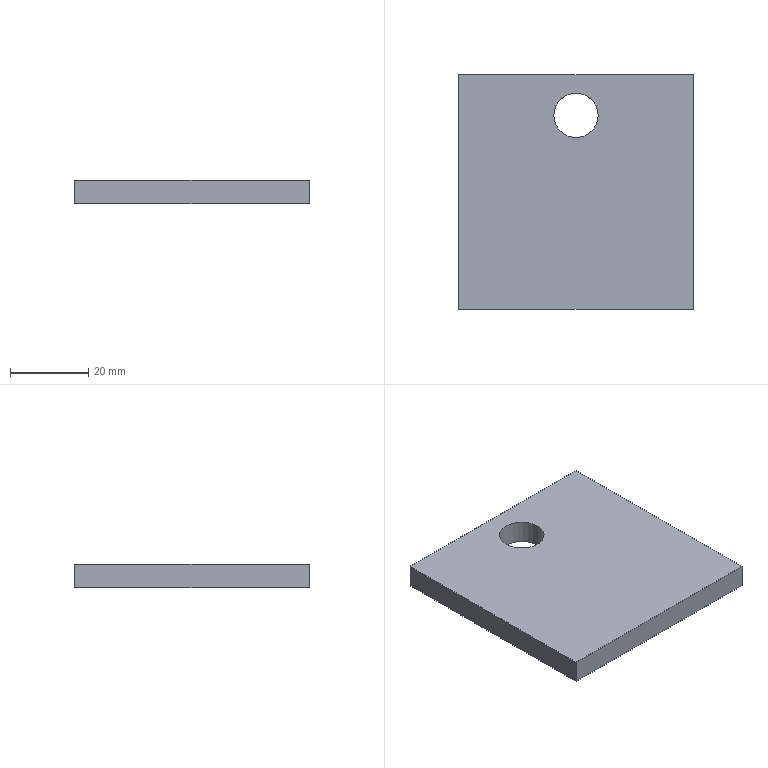Part | NX | features 凸台-拉伸21[1] 2 | 1 solid | 8 faces | box 60 x 60 x 6 mm | volume 20990 mm3 | plane 6 | cylinder 2 | commonest cylinder face diameters 11.377 x2
STEP:
#1=CARTESIAN_POINT('',(2757.312,-550.427,-1102.985));
#2=VERTEX_POINT('',#1);
#3=CARTESIAN_POINT('',(2757.312,-550.427,-1108.985));
#4=VERTEX_POINT('',#3);
#5=CARTESIAN_POINT('',(2757.312,-550.427,-1108.985));
#6=DIRECTION('',(0.,0.,1.));
#7=VECTOR('',#6,1000.);
#8=LINE('',#5,#7);
#9=EDGE_CURVE('',#2,#4,#8,.F.);
#10=ORIENTED_EDGE('',*,*,#9,.T.);
#11=CARTESIAN_POINT('',(2768.688,-550.427,-1108.985));
#12=VERTEX_POINT('',#11);
#13=CARTESIAN_POINT('',(2763.,-550.427,-1108.985));
#14=DIRECTION('',(0.,0.,-1.));
#15=DIRECTION('',(-1.,0.,0.));
#16=AXIS2_PLACEMENT_3D('',#13,#14,#15);
#17=CIRCLE('',#16,5.688);
#18=EDGE_CURVE('',#4,#12,#17,.T.);
#19=ORIENTED_EDGE('',*,*,#18,.T.);
#20=CARTESIAN_POINT('',(2768.688,-550.427,-1102.985));
#21=VERTEX_POINT('',#20);
#22=CARTESIAN_POINT('',(2768.688,-550.427,-1108.985));
#23=DIRECTION('',(0.,0.,1.));
#24=VECTOR('',#23,1000.);
#25=LINE('',#22,#24);
#26=EDGE_CURVE('',#12,#21,#25,.T.);
#27=ORIENTED_EDGE('',*,*,#26,.T.);
#28=CARTESIAN_POINT('',(2763.,-550.427,-1102.985));
#29=DIRECTION('',(0.,0.,-1.));
#30=DIRECTION('',(-1.,0.,0.));
#31=AXIS2_PLACEMENT_3D('',#28,#29,#30);
#32=CIRCLE('',#31,5.688);
#33=EDGE_CURVE('',#2,#21,#32,.T.);
#34=ORIENTED_EDGE('',*,*,#33,.F.);
#35=EDGE_LOOP('',(#10,#19,#27,#34));
#36=FACE_BOUND('',#35,.T.);
#37=CARTESIAN_POINT('',(2763.,-550.427,-1108.985));
#38=DIRECTION('',(0.,0.,1.));
#39=DIRECTION('',(1.,0.,0.));
#40=AXIS2_PLACEMENT_3D('',#37,#38,#39);
#41=CYLINDRICAL_SURFACE('',#40,5.688);
#42=ADVANCED_FACE('',(#36),#41,.F.);
#43=CARTESIAN_POINT('',(2733.,-540.,-1102.985));
#44=VERTEX_POINT('',#43);
#45=CARTESIAN_POINT('',(2793.,-540.,-1102.985));
#46=VERTEX_POINT('',#45);
#47=CARTESIAN_POINT('',(2793.,-540.,-1102.985));
#48=DIRECTION('',(1.,0.,0.));
#49=VECTOR('',#48,1000.);
#50=LINE('',#47,#49);
#51=EDGE_CURVE('',#44,#46,#50,.T.);
#52=ORIENTED_EDGE('',*,*,#51,.T.);
#53=CARTESIAN_POINT('',(2793.,-540.,-1108.985));
#54=VERTEX_POINT('',#53);
#55=CARTESIAN_POINT('',(2793.,-540.,-1108.985));
#56=DIRECTION('',(0.,0.,1.));
#57=VECTOR('',#56,1000.);
#58=LINE('',#55,#57);
#59=EDGE_CURVE('',#54,#46,#58,.T.);
#60=ORIENTED_EDGE('',*,*,#59,.F.);
#61=CARTESIAN_POINT('',(2733.,-540.,-1108.985));
#62=VERTEX_POINT('',#61);
#63=CARTESIAN_POINT('',(2793.,-540.,-1108.985));
#64=DIRECTION('',(1.,0.,0.));
#65=VECTOR('',#64,1000.);
#66=LINE('',#63,#65);
#67=EDGE_CURVE('',#62,#54,#66,.T.);
#68=ORIENTED_EDGE('',*,*,#67,.F.);
#69=CARTESIAN_POINT('',(2733.,-540.,-1108.985));
#70=DIRECTION('',(0.,0.,1.));
#71=VECTOR('',#70,1000.);
#72=LINE('',#69,#71);
#73=EDGE_CURVE('',#62,#44,#72,.T.);
#74=ORIENTED_EDGE('',*,*,#73,.T.);
#75=EDGE_LOOP('',(#52,#60,#68,#74));
#76=FACE_BOUND('',#75,.T.);
#77=CARTESIAN_POINT('',(2793.,-540.,-1108.985));
#78=DIRECTION('',(0.,-1.,0.));
#79=DIRECTION('',(0.,0.,-1.));
#80=AXIS2_PLACEMENT_3D('',#77,#78,#79);
#81=PLANE('',#80);
#82=ADVANCED_FACE('',(#76),#81,.F.);
#83=CARTESIAN_POINT('',(2733.,-600.,-1102.985));
#84=VERTEX_POINT('',#83);
#85=CARTESIAN_POINT('',(2733.,-600.,-1102.985));
#86=DIRECTION('',(0.,1.,0.));
#87=VECTOR('',#86,1000.);
#88=LINE('',#85,#87);
#89=EDGE_CURVE('',#84,#44,#88,.T.);
#90=ORIENTED_EDGE('',*,*,#89,.T.);
#91=ORIENTED_EDGE('',*,*,#73,.F.);
#92=CARTESIAN_POINT('',(2733.,-600.,-1108.985));
#93=VERTEX_POINT('',#92);
#94=CARTESIAN_POINT('',(2733.,-600.,-1108.985));
#95=DIRECTION('',(0.,1.,0.));
#96=VECTOR('',#95,1000.);
#97=LINE('',#94,#96);
#98=EDGE_CURVE('',#93,#62,#97,.T.);
#99=ORIENTED_EDGE('',*,*,#98,.F.);
#100=CARTESIAN_POINT('',(2733.,-600.,-1108.985));
#101=DIRECTION('',(0.,0.,1.));
#102=VECTOR('',#101,1000.);
#103=LINE('',#100,#102);
#104=EDGE_CURVE('',#93,#84,#103,.T.);
#105=ORIENTED_EDGE('',*,*,#104,.T.);
#106=EDGE_LOOP('',(#90,#91,#99,#105));
#107=FACE_BOUND('',#106,.T.);
#108=CARTESIAN_POINT('',(2733.,-600.,-1108.985));
#109=DIRECTION('',(1.,0.,0.));
#110=DIRECTION('',(0.,0.,-1.));
#111=AXIS2_PLACEMENT_3D('',#108,#109,#110);
#112=PLANE('',#111);
#113=ADVANCED_FACE('',(#107),#112,.F.);
#114=CARTESIAN_POINT('',(2793.,-600.,-1102.985));
#115=VERTEX_POINT('',#114);
#116=CARTESIAN_POINT('',(2793.,-600.,-1102.985));
#117=DIRECTION('',(-1.,0.,0.));
#118=VECTOR('',#117,1000.);
#119=LINE('',#116,#118);
#120=EDGE_CURVE('',#115,#84,#119,.T.);
#121=ORIENTED_EDGE('',*,*,#120,.T.);
#122=ORIENTED_EDGE('',*,*,#104,.F.);
#123=CARTESIAN_POINT('',(2793.,-600.,-1108.985));
#124=VERTEX_POINT('',#123);
#125=CARTESIAN_POINT('',(2793.,-600.,-1108.985));
#126=DIRECTION('',(-1.,0.,0.));
#127=VECTOR('',#126,1000.);
#128=LINE('',#125,#127);
#129=EDGE_CURVE('',#124,#93,#128,.T.);
#130=ORIENTED_EDGE('',*,*,#129,.F.);
#131=CARTESIAN_POINT('',(2793.,-600.,-1108.985));
#132=DIRECTION('',(0.,0.,1.));
#133=VECTOR('',#132,1000.);
#134=LINE('',#131,#133);
#135=EDGE_CURVE('',#124,#115,#134,.T.);
#136=ORIENTED_EDGE('',*,*,#135,.T.);
#137=EDGE_LOOP('',(#121,#122,#130,#136));
#138=FACE_BOUND('',#137,.T.);
#139=CARTESIAN_POINT('',(2793.,-600.,-1108.985));
#140=DIRECTION('',(0.,1.,0.));
#141=DIRECTION('',(0.,0.,1.));
#142=AXIS2_PLACEMENT_3D('',#139,#140,#141);
#143=PLANE('',#142);
#144=ADVANCED_FACE('',(#138),#143,.F.);
#145=CARTESIAN_POINT('',(2793.,-600.,-1102.985));
#146=DIRECTION('',(0.,-1.,0.));
#147=VECTOR('',#146,1000.);
#148=LINE('',#145,#147);
#149=EDGE_CURVE('',#46,#115,#148,.T.);
#150=ORIENTED_EDGE('',*,*,#149,.T.);
#151=ORIENTED_EDGE('',*,*,#135,.F.);
#152=CARTESIAN_POINT('',(2793.,-600.,-1108.985));
#153=DIRECTION('',(0.,-1.,0.));
#154=VECTOR('',#153,1000.);
#155=LINE('',#152,#154);
#156=EDGE_CURVE('',#54,#124,#155,.T.);
#157=ORIENTED_EDGE('',*,*,#156,.F.);
#158=ORIENTED_EDGE('',*,*,#59,.T.);
#159=EDGE_LOOP('',(#150,#151,#157,#158));
#160=FACE_BOUND('',#159,.T.);
#161=CARTESIAN_POINT('',(2793.,-600.,-1108.985));
#162=DIRECTION('',(-1.,0.,0.));
#163=DIRECTION('',(0.,0.,1.));
#164=AXIS2_PLACEMENT_3D('',#161,#162,#163);
#165=PLANE('',#164);
#166=ADVANCED_FACE('',(#160),#165,.F.);
#167=CARTESIAN_POINT('',(2763.,-550.427,-1102.985));
#168=DIRECTION('',(0.,0.,-1.));
#169=DIRECTION('',(-1.,0.,0.));
#170=AXIS2_PLACEMENT_3D('',#167,#168,#169);
#171=CIRCLE('',#170,5.688);
#172=EDGE_CURVE('',#21,#2,#171,.T.);
#173=ORIENTED_EDGE('',*,*,#172,.T.);
#174=ORIENTED_EDGE('',*,*,#33,.T.);
#175=EDGE_LOOP('',(#173,#174));
#176=FACE_BOUND('',#175,.T.);
#177=ORIENTED_EDGE('',*,*,#149,.F.);
#178=ORIENTED_EDGE('',*,*,#51,.F.);
#179=ORIENTED_EDGE('',*,*,#89,.F.);
#180=ORIENTED_EDGE('',*,*,#120,.F.);
#181=EDGE_LOOP('',(#177,#178,#179,#180));
#182=FACE_BOUND('',#181,.T.);
#183=CARTESIAN_POINT('',(1500.,0.,-1102.985));
#184=DIRECTION('',(0.,0.,1.));
#185=DIRECTION('',(1.,0.,0.));
#186=AXIS2_PLACEMENT_3D('',#183,#184,#185);
#187=PLANE('',#186);
#188=ADVANCED_FACE('',(#176,#182),#187,.T.);
#189=CARTESIAN_POINT('',(2763.,-550.427,-1108.985));
#190=DIRECTION('',(0.,0.,-1.));
#191=DIRECTION('',(-1.,0.,0.));
#192=AXIS2_PLACEMENT_3D('',#189,#190,#191);
#193=CIRCLE('',#192,5.688);
#194=EDGE_CURVE('',#12,#4,#193,.T.);
#195=ORIENTED_EDGE('',*,*,#194,.F.);
#196=ORIENTED_EDGE('',*,*,#18,.F.);
#197=EDGE_LOOP('',(#195,#196));
#198=FACE_BOUND('',#197,.T.);
#199=ORIENTED_EDGE('',*,*,#156,.T.);
#200=ORIENTED_EDGE('',*,*,#129,.T.);
#201=ORIENTED_EDGE('',*,*,#98,.T.);
#202=ORIENTED_EDGE('',*,*,#67,.T.);
#203=EDGE_LOOP('',(#199,#200,#201,#202));
#204=FACE_BOUND('',#203,.T.);
#205=CARTESIAN_POINT('',(1500.,0.,-1108.985));
#206=DIRECTION('',(0.,0.,1.));
#207=DIRECTION('',(1.,0.,0.));
#208=AXIS2_PLACEMENT_3D('',#205,#206,#207);
#209=PLANE('',#208);
#210=ADVANCED_FACE('',(#198,#204),#209,.F.);
#211=ORIENTED_EDGE('',*,*,#194,.T.);
#212=ORIENTED_EDGE('',*,*,#9,.F.);
#213=ORIENTED_EDGE('',*,*,#172,.F.);
#214=ORIENTED_EDGE('',*,*,#26,.F.);
#215=EDGE_LOOP('',(#211,#212,#213,#214));
#216=FACE_BOUND('',#215,.T.);
#217=CARTESIAN_POINT('',(2763.,-550.427,-1108.985));
#218=DIRECTION('',(0.,0.,1.));
#219=DIRECTION('',(1.,0.,0.));
#220=AXIS2_PLACEMENT_3D('',#217,#218,#219);
#221=CYLINDRICAL_SURFACE('',#220,5.688);
#222=ADVANCED_FACE('',(#216),#221,.F.);
#223=CLOSED_SHELL('',(#42,#82,#113,#144,#166,#188,#210,#222));
#224=MANIFOLD_SOLID_BREP('',#223);
#225=(LENGTH_UNIT()NAMED_UNIT(*)SI_UNIT(.MILLI.,.METRE.));
#226=UNCERTAINTY_MEASURE_WITH_UNIT(LENGTH_MEASURE(0.00001),#225,'','');
#227=(NAMED_UNIT(*)PLANE_ANGLE_UNIT()SI_UNIT($,.RADIAN.));
#228=(NAMED_UNIT(*)SI_UNIT($,.STERADIAN.)SOLID_ANGLE_UNIT());
#229=(GEOMETRIC_REPRESENTATION_CONTEXT(3)GLOBAL_UNCERTAINTY_ASSIGNED_CONTEXT((#226))GLOBAL_UNIT_ASSIGNED_CONTEXT((#225,#227,#228))REPRESENTATION_CONTEXT('',''));
#230=ADVANCED_BREP_SHAPE_REPRESENTATION('',(#224),#229);